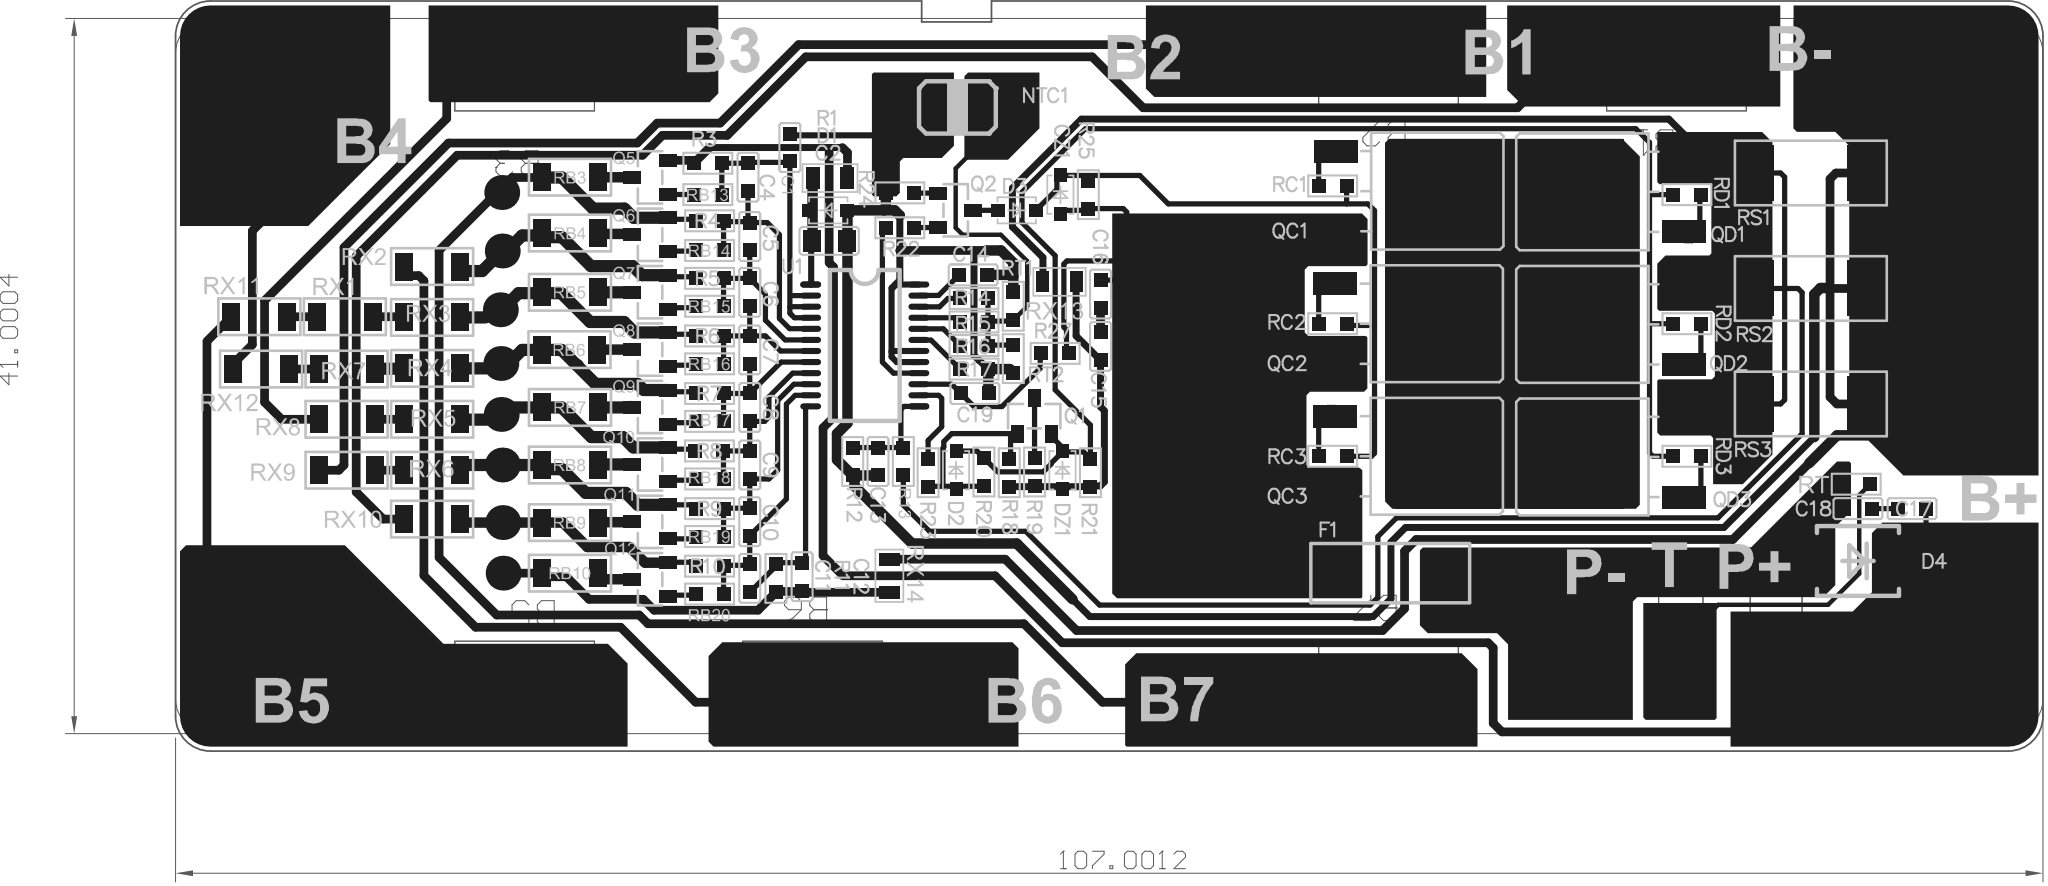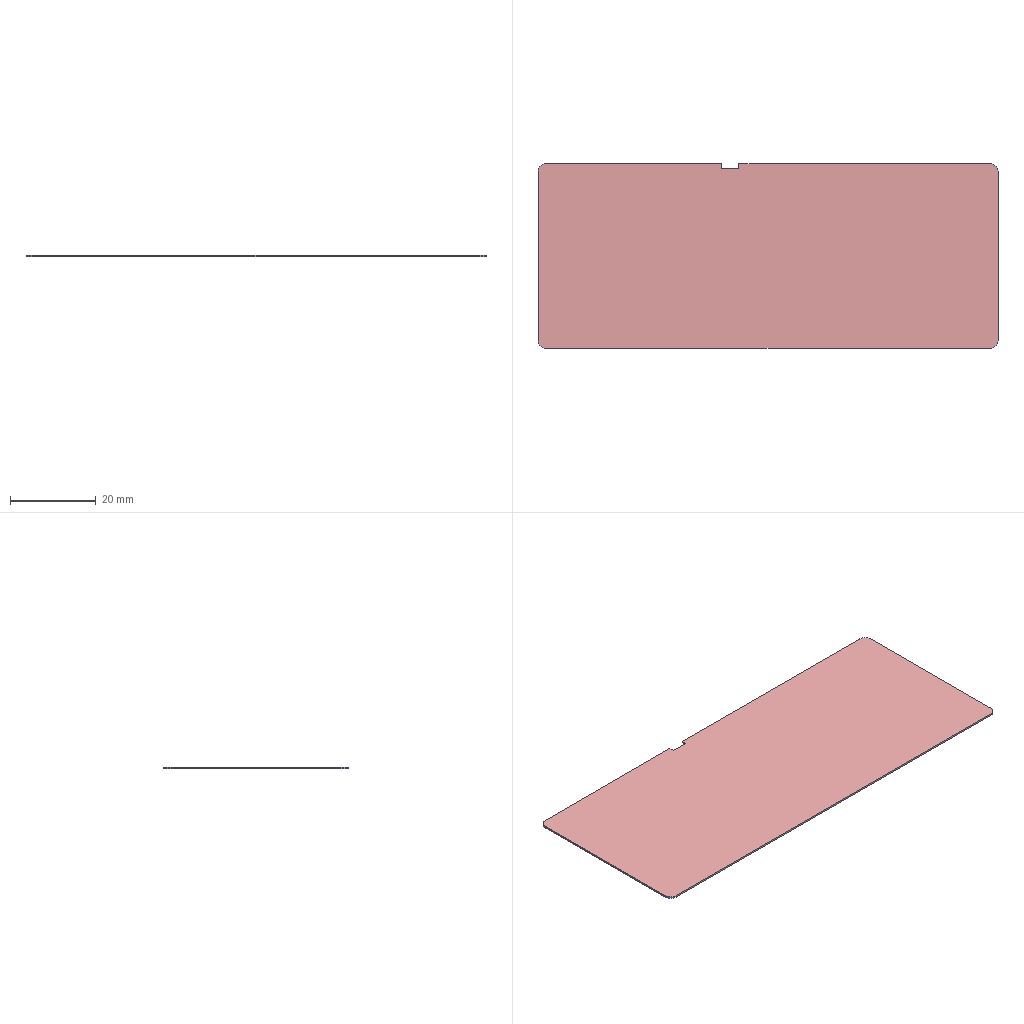Circuit board layout | Altium Designer | box 107 x 43 x 0.4 mm
Layer stack:
# Altium Designer layer stack of  (unit mm; dielectric type: 0 none, 1 core, 2 prepreg, 3 surface material)
index,name,kind,layer,copper_thickness_mm,dielectric_type,dielectric_thickness_mm,dielectric_material,dielectric_constant
0,Top Paste,other,,,,,,
1,Top Overlay,other,,,,,,
2,Top Solder,dielectric,,,3,0.0102,Solder Resist,3.5
3,Top Layer,copper,Top Layer,0.0356,,,,
4,Dielectric 1,dielectric,,,0,0.32,FR-4,4.8
5,Bottom Layer,copper,Bottom Layer,0.0356,,,,
6,Bottom Solder,dielectric,,,3,0.0102,Solder Resist,3.5
7,Bottom Overlay,other,,,,,,
8,Bottom Paste,other,,,,,,
# drill layer pairs: low layer,high layer
drill_pair,Top Layer,Bottom Layer
Part placement:
Designator,Comment,Layer,Footprint,Center-X(mm),Center-Y(mm),Rotation
RX14,1K,TopLayer,R0805A,38.9,-29.95,90
RX13,1K,TopLayer,R0805A,48.65,-13.1,180
RX12,1K,TopLayer,R1206A,2.9,-18.1,180
RX11,1K,TopLayer,R1206A,2.8,-15.1,180
RX10,1K,TopLayer,R1206A,12.7,-26.7,0
RX9,1K,TopLayer,R1206A,7.8,-23.9,0
RX8,1K,TopLayer,R1206A,7.8,-20.98,0
RX7,1K,TopLayer,R1206A,7.8,-18.1,180
RX6,1K,TopLayer,R1206A,12.7,-23.9,180
RX5,1K,TopLayer,R1206A,12.7,-20.98,180
RX4,1K,TopLayer,R1206A,12.7,-18.06,180
RX3,1K,TopLayer,R1206A,12.7,-15.14,180
RX2,1K,TopLayer,R1206A,12.7,-12.22,180
RX1,1K,TopLayer,R1206A,7.7,-15.1,180
RT,1K,TopLayer,R0603A,94.3,-24.7,0
T,Pad,TopLayer,Pad10X8mm,84.019,-34.617,90
R13,1K,TopLayer,R0603A,39.7,-23.4,270
RB20,1K,TopLayer,R0603A,28.6,-31,0
RB19,1K,TopLayer,R0603A,28.6,-27.7,0
RB18,1K,TopLayer,R0603A,28.6,-24.4,0
RB17,1K,TopLayer,R0603A,28.6,-21.1,0
RB16,1K,TopLayer,R0603A,28.6,-17.8,0
RB15,1K,TopLayer,R0603A,28.6,-14.5,0
RB14,1K,TopLayer,R0603A,28.6,-11.3,0
RB13,1K,TopLayer,R0603A,28.5,-8.1,0
RB10,51R,TopLayer,R1206A,20.6,-29.8,0
RB9,51R,TopLayer,R1206A,20.6,-26.9,0
RB8,51R,TopLayer,R1206A,20.6,-23.6,0
RB7,51R,TopLayer,R1206A,20.6,-20.3,0
RB6,51R,TopLayer,R1206A,20.573,-16.984,0
RB5,51R,TopLayer,R1206A,20.6,-13.7,0
RB4,51R,TopLayer,R1206A,20.6,-10.3,0
RB3,51R,TopLayer,R1206A,20.6,-7.1,0
Q12,MMBT5401,TopLayer,SOT23-3,25.181,-30.15,90
Q11,MMBT5401,TopLayer,SOT23-3,25.181,-26.858,90
Q10,MMBT5401,TopLayer,SOT23-3,25.181,-23.567,90
Q9,MMBT5401,TopLayer,SOT23-3,25.181,-20.275,90
Q8,MMBT5401,TopLayer,SOT23-3,25.181,-16.984,90
Q7,MMBT5401,TopLayer,SOT23-3,25.181,-13.692,90
Q6,MMBT5401,TopLayer,SOT23-3,25.181,-10.401,90
Q5,MMBT5401,TopLayer,SOT23-3,25.181,-7.109,90
C1,0.1uF,TopLayer,C0603A,33.2,-5.4,270
U1,CW1104/ERP2018,TopLayer,TSSOP-24(pin间距0.635mm),37.491,-16.746,0
R12,1K,TopLayer,R0603A,36.8,-23.4,90
RT1,1K,TopLayer,R0603A,46,-14.5,90
RT2,1K,TopLayer,R0603A,46,-17.5,270
RS3,R010,TopLayer,R2512L,91.7,-20.1,180
RS2,R010,TopLayer,R2512L,91.7,-13.479,180
RS1,R010,TopLayer,R2512L,91.7,-6.859,180
R27,1K,TopLayer,R0603A,48.4,-17.2,180
RC3,1K,TopLayer,R0603A,64.3,-23.1,180
RC2,1K,TopLayer,R0603A,64.3,-15.5,180
R25,1K,TopLayer,R0603A,50.3,-8.1,270
RC1,1K,TopLayer,R0603A,64.3,-7.6,0
R24,1K,TopLayer,R0603A,39.5,-8,180
RD1,1K,TopLayer,R0603A,84.6,-8.1,180
R23,1K,TopLayer,R0603A,41.12,-24.042,270
RD3,1K,TopLayer,R0603A,84.6,-23.1,180
RD2,1K,TopLayer,R0603A,84.6,-15.5,180
R22,1K,TopLayer,R0603A,39.5,-10,0
R21,1K,TopLayer,R0603A,50.42,-24.042,270
R20,1K,TopLayer,R0603A,44.32,-24,90
R19,1K,TopLayer,R0603A,47.22,-24,270
R18,1K,TopLayer,R0603A,45.77,-24.042,270
R17,1K,TopLayer,R0603A,43.75,-18.1,0
R16,1K,TopLayer,R0603A,43.75,-16.75,0
R15,1K,TopLayer,R0603A,43.75,-15.4,0
R14,1K,TopLayer,R0603A,43.75,-14.05,0
R11,1K,TopLayer,R0603A,32.4,-30.1,90
R10,1K,TopLayer,R0603A,28.6,-29.4,0
R9,1K,TopLayer,R0603A,28.6,-26.1,0
R8,1K,TopLayer,R0603A,28.589,-22.792,0
R7,1K,TopLayer,R0603A,28.6,-19.5,0
R6,1K,TopLayer,R0603A,28.6,-16.2,0
R5,1K,TopLayer,R0603A,28.6,-12.9,0
R4,1K,TopLayer,R0603A,28.6,-9.6,0
R3,1K,TopLayer,R0603A,28.5,-6.3,0
R1,100R/1K*0805,TopLayer,R0805A,35.5,-7.15,180
QD3,TO-252 N MOS*,TopLayer,TO-252,81.219,-23.139,90
QD2,TO-252 N MOS*,TopLayer,TO-252,81.219,-15.539,90
QD1,TO-252 N MOS*,TopLayer,TO-252,81.219,-7.939,90
Q2,MMBT5401,TopLayer,SOT23-3,42.708,-9,270
QC3,TO-252 N MOS*,TopLayer,TO-252,67.656,-23.1,270
QC2,TO-252 N MOS*,TopLayer,TO-252,67.656,-15.5,270
QC1,TO-252 N MOS*,TopLayer,TO-252,67.688,-7.9,270
Q1,MMBT5401/N*,TopLayer,SOT23-3,47.2,-20.792,0
P-,Pad,TopLayer,Pad10X8mm,78.802,-34.422,270
P+,Pad,TopLayer,Pad10X8mm,89.722,-34.422,270
NTC1,10K B=3435,TopLayer,RT2.3X1.2-2,42.8,-3.1,180
F1,F2410 60V30A,TopLayer,F2410,67.6,-29.8,0
DZ1,15V,TopLayer,SOD323,48.82,-23.9,270
D4,RS3M,TopLayer,SMB(DO-214AA),94.4,-29.1,180
D3,1N4148SW,TopLayer,SOD323,46.2,-9,180
D2,1N4148SW/NC*,TopLayer,SOD323,42.72,-23.9,270
D1,56V,TopLayer,SOD323,35.4,-9,0
CZ1,15V,TopLayer,SOD323,48.7,-8.1,270
C18,0.1uF,TopLayer,C0603A,94.4,-26.1,0
C17,0.1uF,TopLayer,C0603A,97.5,-26.1,0
C19,0.01uF/NC*,TopLayer,C0603A,43.8,-19.5,0
C16,0.1uF,TopLayer,C0603A,51,-13.8,270
C15,0.1uF,TopLayer,C0603A,51,-16.8,270
C14,0.1uF/NC*,TopLayer,C0603A,43.7,-12.7,180
C13,0.1uF,TopLayer,C0603A,38.25,-23.4,90
C12,1uF/NC*,TopLayer,C0603A,33.9,-30,90
C11,0.1uF,TopLayer,C0603A,30.9,-30.1,90
C10,0.1uF,TopLayer,C0603A,30.9,-26.85,90
C9,0.1uF,TopLayer,C0603A,30.9,-23.6,90
C8,0.1uF,TopLayer,C0603A,30.9,-20.3,90
C7,0.1uF,TopLayer,C0603A,30.9,-17,90
C6,0.1uF,TopLayer,C0603A,30.9,-13.7,90
C5,0.1uF,TopLayer,C0603A,30.9,-10.5,90
C4,0.1uF,TopLayer,C0603A,30.8,-7.1,90
C2,1uF50V/0805,TopLayer,C0805A,35.45,-10.75,180
B-,Pad,TopLayer,Pad10X8mm,97.501,0.2,90
B+,Pad,TopLayer,Pad10X8mm,97.501,-37.2,270
B7,Pad,TopLayer,Pad10X8mm,67.501,-37.2,270
B6,Pad,TopLayer,Pad10X8mm,34.5,-37.2,270
B5,Pad,TopLayer,Pad10X8mm,18,-37.206,270
B4,Pad,TopLayer,Pad10X8mm,5.5,0.2,270
B3,Pad,TopLayer,Pad10X8mm,18,0.2,270
B2,Pad,TopLayer,Pad10X8mm,67.501,0.2,270
B1,Pad,TopLayer,Pad10X8mm,84.001,0.1939,270
Pad and via stacks:
# Altium Designer via and pad stacks of  (unit mm). Each distinct definition once, with the count of objects using it.
# via: kind,start_layer,end_layer,hole_mm,diameter_mm,mode(0 simple;1 top-mid-bottom;2 full stack),diameter_per_layer,count,example_net
# pad: kind,layer,hole_mm,hole_type(0 round;1 square;2 slot),plating,top_size,top_shape(1 round;2 rect;3 octagon;9 rounded rect),mid_size,bottom_size,mode,footprint,size_per_layer,count,example
pad,Top Layer,0,0,plated,2x2,1,2x2,2x2,0,,,8,10
pad,Top Layer,0,0,plated,1x1.6,2,1x1.6,1x1.6,0,R1206A,,40,RB3.1
pad,Top Layer,0,2,plated,4.6x3,2,4.6x3,4.6x3,0,Pad10X8mm,,2,P-.1
pad,Top Layer,0,2,plated,5x8,2,5x8,5x8,0,Pad10X8mm,,9,B7.1
pad,Top Layer,0,2,plated,4x3,2,4x3,4x3,0,Pad10X8mm,,1,T.1
pad,Top Layer,0,0,plated,0.8x0.8,2,0.8x0.8,0.8x0.8,0,R0603A,,82,RT.1
pad,Top Layer,0,0,plated,2x2.5,2,2x2.5,2x2.5,0,SMB(DO-214AA),,2,D4.1
pad,Top Layer,0,0,plated,0.8x0.8,2,0.8x0.8,0.8x0.8,0,C0603A,,34,C17.1
pad,Top Layer,0,2,plated,3x3,1,3x3,3x3,0,,,12,8
pad,Top Layer,0,2,plated,0.8x0.8,1,0.8x0.8,0.8x0.8,0,,,2,2
pad,Top Layer,0,0,plated,1.3x2.5,2,1.3x2.5,1.3x2.5,0,TO-252,,12,QC2.1
pad,Top Layer,0,0,plated,6x6,2,6x6,6x6,0,TO-252,,6,QC2.3
pad,Top Layer,0,0,plated,0.7x1.2,2,0.7x1.2,0.7x1.2,0,R0805A,,4,RX14.2
pad,Top Layer,0,2,plated,2.8x2.5,2,2.8x2.5,2.8x2.5,0,F2410,,2,F1.2
pad,Top Layer,0,0,plated,0.7x1,2,0.7x1,0.7x1,0,SOT23-3,,30,Q12.1
pad,Top Layer,0,0,plated,2x3.2,2,2x3.2,2x3.2,0,R2512L,,6,RS3.1
pad,Top Layer,0,0,plated,0.8x0.7,2,0.8x0.7,0.8x0.7,0,SOD323,,10,DZ1.2
pad,Top Layer,0,0,plated,1.2x2.3,1,1.2x2.3,1.2x2.3,0,RT2.3X1.2-2,,2,NTC1.1
pad,Top Layer,0,0,plated,1.2x0.35,1,1.2x0.35,1.2x0.35,0,TSSOP-24(pin\u00BC\u00E4\u00BE\u00E00.635mm),,26,U1.21
pad,Top Layer,0,0,plated,1x1.25,2,1x1.25,1x1.25,0,C0805A,,2,C2.1
pad,Top Layer,0,0,plated,0.8x1.25,2,0.8x1.25,0.8x1.25,0,R0805A,,2,R1.2
pad,Top Solder,0,0,plated,2.5x20,2,2.5x20,2.5x20,0,,,4,9
Copper pours:
name,layer,net,type(0 solid;1 hatched;2 none)
NONET_L02_P-001,Top Layer,B1,0
NONET_L02_P-001,Top Layer,P-,0
NONET_L02_P-001,Top Layer,B7,0
NONET_L02_P-001,Top Layer,B-,0
NONET_L02_P-001,Top Layer,NetNTC1_1,0
NONET_L02_P-001,Top Layer,NetC16_1,0
NONET_L02_P-001,Top Layer,B3,0
NONET_L02_P-001,Top Layer,T,0
NONET_L02_P-001,Top Layer,B2,0
NONET_L02_P-001,Top Layer,NetQC1_3,0
NONET_L02_P-001,Top Layer,B6,0
NONET_L02_P-001,Top Layer,B5,0
NONET_L02_P-001,Top Layer,B4,0
NONET_L02_P-001,Top Layer,B+,0
NONET_L02_P-001,Top Layer,CS,0
NONET_L02_P-001,Top Layer,B-,0
Design rules, without the lines most boards share:
# Altium Designer design rules of  (exported by Altium Designer, unit mm)
# columns: name | kind | enabled | priority | scope1 | scope2 | descriptor | typed fields (field=value)
Schematic Supply Nets_1 | 41 | enabled | 1 | InNet('B-') | All | Supply Net(s)(InNet('B-')) |
Schematic Supply Nets | 41 | enabled | 2 | InNet('P-') | All | Supply Net(s)(InNet('P-')) |
NetAntennae | 56 | enabled | 1 | All | All | Net Antennae (Tolerance=0mm) (All) |
SilkToSilkClearance | 55 | enabled | 1 | All | All | Silk to Silk (Clearance=0mm) (All),(All) |
SilkToSolderMaskClearance | 54 | enabled | 1 | IsPad | All | Silk To Solder Mask (Clearance=0mm) (IsPad),(All) |
MinimumSolderMaskSliver | 53 | enabled | 1 | All | All | Minimum Solder Mask Sliver (Gap=0mm) (All),(All) |
HoleToHoleClearance | 52 | enabled | 1 | All | All | Hole To Hole Clearance (Gap=0mm) (All),(All) | gap=0
DiffPairsRouting | 51 | enabled | 1 | All | All | Differential Pairs Uncoupled Length using the Gap Constraints (Min=0.254mm) (Max=0.254mm) (Prefered=0.254mm)  and Width Constraints (Min=0.381mm) (Max=0.381mm) (Prefered=0.381mm) (All) |
HoleSize | 42 | enabled | 1 | All | All | Hole Size Constraint (Min=0.025mm) (Max=2.54mm) (All) |
Height | 50 | enabled | 1 | All | All | Height Constraint (Min=0mm) (Max=25.4mm) (Prefered=12.7mm) (All) | min_height=0 max_height=25.4
ComponentClearance | 24 | enabled | 1 | All | All | Component Clearance Constraint ( Horizontal Gap = 0mm, Vertical Gap = 0mm ) (All),(All)  | gap=0
SolderMaskExpansion | 13 | enabled | 1 | All | All | Solder Mask Expansion (Expansion =0.102mm) (All) | expansion=0.1016
PasteMaskExpansion | 14 | enabled | 1 | All | All | Paste Mask Expansion (Expansion =0mm) (All) | expansion=0
RoutingVias | 11 | enabled | 1 | All | All | Routing Via (MinHoleWidth=0.4mm) (MaxHoleWidth=0.4mm) (PreferredHoleWidth=0.4mm) (MinWidth=0.6mm) (MaxWidth=0.6mm) (PreferedWidth=0.6mm) (All) | via_min_hole=0.4 via_max_hole=0.4 via_preferred_diameter=0.6 via_preferred_hole=0.4
RoutingCorners | 10 | enabled | 1 | All | All | Routing Corners (Style=45-Degree) (Min Setback=2.54mm) (Max Setback=2.54mm) (All) |
Width | 2 | enabled | 1 | All | All | Width Constraint (Min=0.254mm) (Max=1mm) (Preferred=0.254mm) (All) |
PolygonConnect | 20 | enabled | 1 | All | All | Polygon Connect Rule(Direct Connect )(Conductor Width=0.254mm) (Relief Angle=90 Angle) (Entries=4) (Air Gap Width=0.254mm) (All),(All) | connect_style(0=relief,1=direct,2=none)=1 relief_conductor_width=0.254 relief_entries=4
PlaneClearance | 12 | enabled | 1 | All | All | Power Plane Clearance (Clearance =0.508mm) (All) | clearance=0.508
PlaneConnect | 6 | enabled | 1 | All | All | Power Plane Connect Rule(Direct Connect )(Expansion=0.508mm) (Conductor Width=0.254mm) (Air Gap=0.254mm) (Entries=4) (All) | relief_conductor_width=0.254 relief_entries=4 relief_expansion=0.508
Clearance | 0 | enabled | 1 | All | All | Clearance Constraint (Gap=0.2mm) (All),(All) | gap=0.2